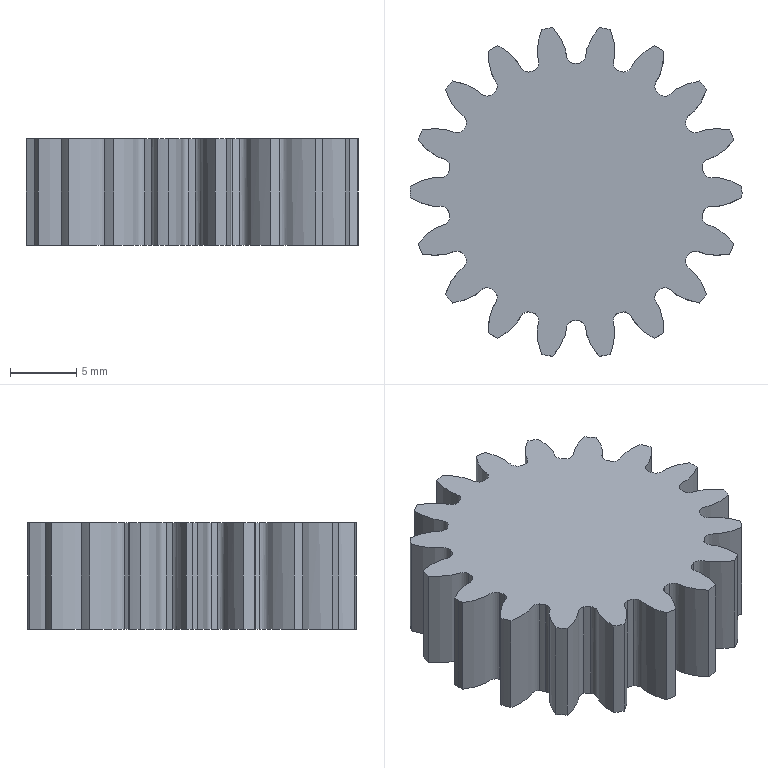Part | SolidWorks | features CirPattern 1, Extrusion 1, ICE 1, RefAxis 1 | 1 solid | 75 faces | box 25 x 24.753 x 8 mm | volume 3124 mm3 | cylinder 37 | spline 36 | plane 2 | commonest cylinder face diameters 25 x19 19.375 x18